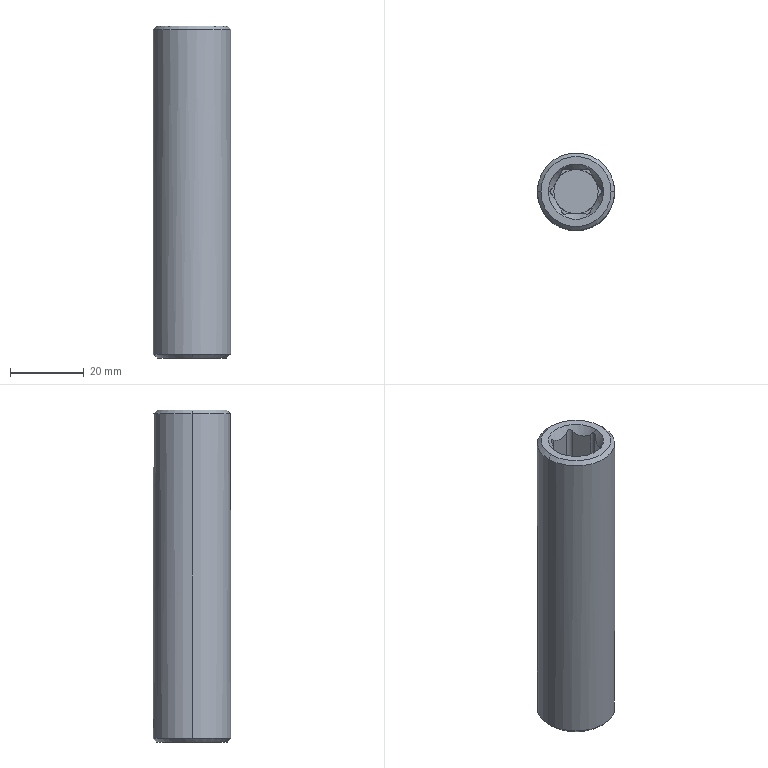Part | STEP file | Hex head-PN_0001 | 1 solid | 49 faces | box 21 x 21 x 90 mm | volume 27340 mm3 | plane 24 | cylinder 19 | cone 6 | commonest cylinder face diameters 2 x13 3.5 x2 12 x2 21 x2